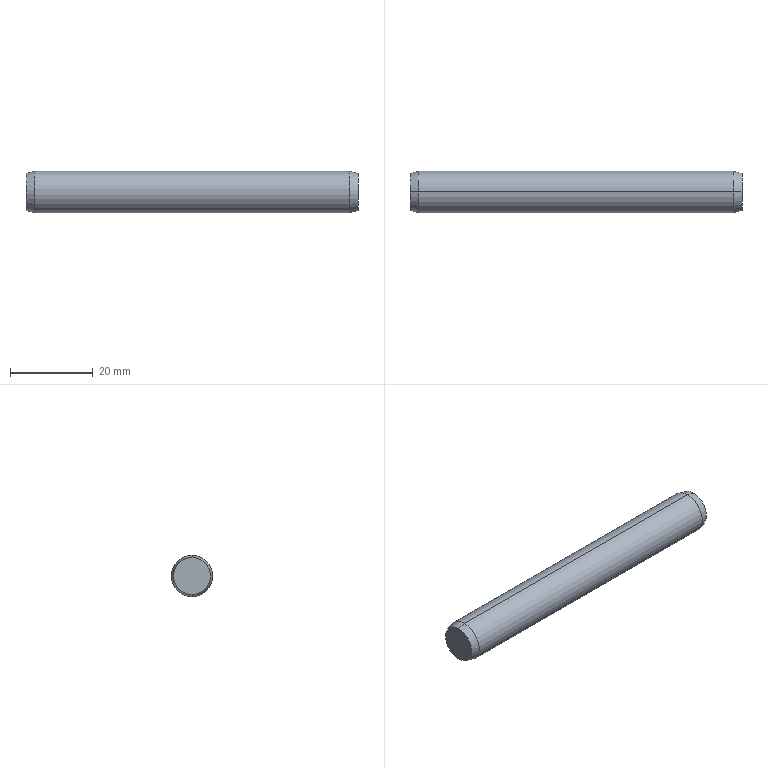Part | SolidWorks | features Revolution 1 | 1 solid | 8 faces | box 80 x 10 x 10 mm | volume 6251 mm3 | cone 4 | cylinder 2 | plane 2 | commonest cylinder face diameters 10 x2
STEP:
#1=CARTESIAN_POINT('',(0.,0.,-4.464));
#2=VERTEX_POINT('',#1);
#3=CARTESIAN_POINT('',(0.,0.,4.464));
#4=VERTEX_POINT('',#3);
#5=CARTESIAN_POINT('',(0.,0.,0.));
#6=DIRECTION('',(1.,0.,0.));
#7=DIRECTION('',(0.,0.,-1.));
#8=AXIS2_PLACEMENT_3D('',#5,#6,#7);
#9=CIRCLE('',#8,4.464);
#10=EDGE_CURVE('',#2,#4,#9,.T.);
#11=ORIENTED_EDGE('',*,*,#10,.T.);
#12=CARTESIAN_POINT('',(2.,0.,5.));
#13=VERTEX_POINT('',#12);
#14=CARTESIAN_POINT('',(2.,0.,5.));
#15=DIRECTION('',(0.9659,0.,0.2588));
#16=VECTOR('',#15,1000.);
#17=LINE('',#14,#16);
#18=EDGE_CURVE('',#4,#13,#17,.T.);
#19=ORIENTED_EDGE('',*,*,#18,.T.);
#20=CARTESIAN_POINT('',(2.,0.,-5.));
#21=VERTEX_POINT('',#20);
#22=CARTESIAN_POINT('',(2.,0.,0.));
#23=DIRECTION('',(1.,0.,0.));
#24=DIRECTION('',(0.,0.,-1.));
#25=AXIS2_PLACEMENT_3D('',#22,#23,#24);
#26=CIRCLE('',#25,5.);
#27=EDGE_CURVE('',#21,#13,#26,.T.);
#28=ORIENTED_EDGE('',*,*,#27,.F.);
#29=CARTESIAN_POINT('',(2.,0.,-5.));
#30=DIRECTION('',(0.9659,0.,-0.2588));
#31=VECTOR('',#30,1000.);
#32=LINE('',#29,#31);
#33=EDGE_CURVE('',#2,#21,#32,.T.);
#34=ORIENTED_EDGE('',*,*,#33,.F.);
#35=EDGE_LOOP('',(#11,#19,#28,#34));
#36=FACE_OUTER_BOUND('',#35,.T.);
#37=CARTESIAN_POINT('',(2.,0.,0.));
#38=DIRECTION('',(1.,0.,0.));
#39=DIRECTION('',(0.,0.,-1.));
#40=AXIS2_PLACEMENT_3D('',#37,#38,#39);
#41=CONICAL_SURFACE('',#40,5.,0.2618);
#42=ADVANCED_FACE('',(#36),#41,.T.);
#43=ORIENTED_EDGE('',*,*,#27,.T.);
#44=CARTESIAN_POINT('',(78.,0.,5.));
#45=VERTEX_POINT('',#44);
#46=CARTESIAN_POINT('',(0.,0.,5.));
#47=DIRECTION('',(1.,0.,0.));
#48=VECTOR('',#47,1000.);
#49=LINE('',#46,#48);
#50=EDGE_CURVE('',#13,#45,#49,.T.);
#51=ORIENTED_EDGE('',*,*,#50,.T.);
#52=CARTESIAN_POINT('',(78.,0.,-5.));
#53=VERTEX_POINT('',#52);
#54=CARTESIAN_POINT('',(78.,0.,0.));
#55=DIRECTION('',(1.,0.,0.));
#56=DIRECTION('',(0.,0.,-1.));
#57=AXIS2_PLACEMENT_3D('',#54,#55,#56);
#58=CIRCLE('',#57,5.);
#59=EDGE_CURVE('',#53,#45,#58,.T.);
#60=ORIENTED_EDGE('',*,*,#59,.F.);
#61=CARTESIAN_POINT('',(0.,0.,-5.));
#62=DIRECTION('',(1.,0.,0.));
#63=VECTOR('',#62,1000.);
#64=LINE('',#61,#63);
#65=EDGE_CURVE('',#21,#53,#64,.T.);
#66=ORIENTED_EDGE('',*,*,#65,.F.);
#67=EDGE_LOOP('',(#43,#51,#60,#66));
#68=FACE_OUTER_BOUND('',#67,.T.);
#69=CARTESIAN_POINT('',(0.,0.,0.));
#70=DIRECTION('',(1.,0.,0.));
#71=DIRECTION('',(0.,0.,-1.));
#72=AXIS2_PLACEMENT_3D('',#69,#70,#71);
#73=CYLINDRICAL_SURFACE('',#72,5.);
#74=ADVANCED_FACE('',(#68),#73,.T.);
#75=CARTESIAN_POINT('',(80.,0.,-4.464));
#76=VERTEX_POINT('',#75);
#77=CARTESIAN_POINT('',(80.,0.,4.464));
#78=VERTEX_POINT('',#77);
#79=CARTESIAN_POINT('',(80.,0.,0.));
#80=DIRECTION('',(1.,0.,0.));
#81=DIRECTION('',(0.,0.,-1.));
#82=AXIS2_PLACEMENT_3D('',#79,#80,#81);
#83=CIRCLE('',#82,4.464);
#84=EDGE_CURVE('',#76,#78,#83,.T.);
#85=ORIENTED_EDGE('',*,*,#84,.F.);
#86=CARTESIAN_POINT('',(80.,0.,-4.464));
#87=DIRECTION('',(-0.9659,0.,-0.2588));
#88=VECTOR('',#87,1000.);
#89=LINE('',#86,#88);
#90=EDGE_CURVE('',#76,#53,#89,.T.);
#91=ORIENTED_EDGE('',*,*,#90,.T.);
#92=ORIENTED_EDGE('',*,*,#59,.T.);
#93=CARTESIAN_POINT('',(80.,0.,4.464));
#94=DIRECTION('',(-0.9659,0.,0.2588));
#95=VECTOR('',#94,1000.);
#96=LINE('',#93,#95);
#97=EDGE_CURVE('',#78,#45,#96,.T.);
#98=ORIENTED_EDGE('',*,*,#97,.F.);
#99=EDGE_LOOP('',(#85,#91,#92,#98));
#100=FACE_OUTER_BOUND('',#99,.T.);
#101=CARTESIAN_POINT('',(80.,0.,0.));
#102=DIRECTION('',(-1.,0.,0.));
#103=DIRECTION('',(0.,0.,1.));
#104=AXIS2_PLACEMENT_3D('',#101,#102,#103);
#105=CONICAL_SURFACE('',#104,4.464,0.2618);
#106=ADVANCED_FACE('',(#100),#105,.T.);
#107=ORIENTED_EDGE('',*,*,#10,.F.);
#108=CARTESIAN_POINT('',(0.,0.,0.));
#109=DIRECTION('',(1.,0.,0.));
#110=DIRECTION('',(0.,0.,-1.));
#111=AXIS2_PLACEMENT_3D('',#108,#109,#110);
#112=CIRCLE('',#111,4.464);
#113=EDGE_CURVE('',#4,#2,#112,.T.);
#114=ORIENTED_EDGE('',*,*,#113,.F.);
#115=EDGE_LOOP('',(#107,#114));
#116=FACE_OUTER_BOUND('',#115,.T.);
#117=CARTESIAN_POINT('',(0.,4.464,0.));
#118=DIRECTION('',(-1.,0.,0.));
#119=DIRECTION('',(0.,0.,1.));
#120=AXIS2_PLACEMENT_3D('',#117,#118,#119);
#121=PLANE('',#120);
#122=ADVANCED_FACE('',(#116),#121,.T.);
#123=CARTESIAN_POINT('',(80.,0.,0.));
#124=DIRECTION('',(1.,0.,0.));
#125=DIRECTION('',(0.,0.,-1.));
#126=AXIS2_PLACEMENT_3D('',#123,#124,#125);
#127=CIRCLE('',#126,4.464);
#128=EDGE_CURVE('',#78,#76,#127,.T.);
#129=ORIENTED_EDGE('',*,*,#128,.T.);
#130=ORIENTED_EDGE('',*,*,#84,.T.);
#131=EDGE_LOOP('',(#129,#130));
#132=FACE_OUTER_BOUND('',#131,.T.);
#133=CARTESIAN_POINT('',(80.,4.464,0.));
#134=DIRECTION('',(1.,0.,0.));
#135=DIRECTION('',(0.,0.,-1.));
#136=AXIS2_PLACEMENT_3D('',#133,#134,#135);
#137=PLANE('',#136);
#138=ADVANCED_FACE('',(#132),#137,.T.);
#139=ORIENTED_EDGE('',*,*,#90,.F.);
#140=ORIENTED_EDGE('',*,*,#128,.F.);
#141=ORIENTED_EDGE('',*,*,#97,.T.);
#142=CARTESIAN_POINT('',(78.,0.,0.));
#143=DIRECTION('',(1.,0.,0.));
#144=DIRECTION('',(0.,0.,-1.));
#145=AXIS2_PLACEMENT_3D('',#142,#143,#144);
#146=CIRCLE('',#145,5.);
#147=EDGE_CURVE('',#45,#53,#146,.T.);
#148=ORIENTED_EDGE('',*,*,#147,.T.);
#149=EDGE_LOOP('',(#139,#140,#141,#148));
#150=FACE_OUTER_BOUND('',#149,.T.);
#151=CARTESIAN_POINT('',(80.,0.,0.));
#152=DIRECTION('',(-1.,0.,0.));
#153=DIRECTION('',(0.,0.,1.));
#154=AXIS2_PLACEMENT_3D('',#151,#152,#153);
#155=CONICAL_SURFACE('',#154,4.464,0.2618);
#156=ADVANCED_FACE('',(#150),#155,.T.);
#157=ORIENTED_EDGE('',*,*,#50,.F.);
#158=CARTESIAN_POINT('',(2.,0.,0.));
#159=DIRECTION('',(1.,0.,0.));
#160=DIRECTION('',(0.,0.,-1.));
#161=AXIS2_PLACEMENT_3D('',#158,#159,#160);
#162=CIRCLE('',#161,5.);
#163=EDGE_CURVE('',#13,#21,#162,.T.);
#164=ORIENTED_EDGE('',*,*,#163,.T.);
#165=ORIENTED_EDGE('',*,*,#65,.T.);
#166=ORIENTED_EDGE('',*,*,#147,.F.);
#167=EDGE_LOOP('',(#157,#164,#165,#166));
#168=FACE_OUTER_BOUND('',#167,.T.);
#169=CARTESIAN_POINT('',(0.,0.,0.));
#170=DIRECTION('',(1.,0.,0.));
#171=DIRECTION('',(0.,0.,-1.));
#172=AXIS2_PLACEMENT_3D('',#169,#170,#171);
#173=CYLINDRICAL_SURFACE('',#172,5.);
#174=ADVANCED_FACE('',(#168),#173,.T.);
#175=ORIENTED_EDGE('',*,*,#18,.F.);
#176=ORIENTED_EDGE('',*,*,#113,.T.);
#177=ORIENTED_EDGE('',*,*,#33,.T.);
#178=ORIENTED_EDGE('',*,*,#163,.F.);
#179=EDGE_LOOP('',(#175,#176,#177,#178));
#180=FACE_OUTER_BOUND('',#179,.T.);
#181=CARTESIAN_POINT('',(2.,0.,0.));
#182=DIRECTION('',(1.,0.,0.));
#183=DIRECTION('',(0.,0.,-1.));
#184=AXIS2_PLACEMENT_3D('',#181,#182,#183);
#185=CONICAL_SURFACE('',#184,5.,0.2618);
#186=ADVANCED_FACE('',(#180),#185,.T.);
#187=CLOSED_SHELL('',(#42,#74,#106,#122,#138,#156,#174,#186));
#188=MANIFOLD_SOLID_BREP('',#187);
#189=CARTESIAN_POINT('',(0.,0.,0.));
#190=DIRECTION('',(0.,0.,1.));
#191=DIRECTION('',(1.,0.,0.));
#192=AXIS2_PLACEMENT_3D('',#189,#190,#191);
#193=(LENGTH_UNIT()NAMED_UNIT(*)SI_UNIT(.MILLI.,.METRE.));
#194=UNCERTAINTY_MEASURE_WITH_UNIT(LENGTH_MEASURE(0.00001),#193,'','');
#195=(NAMED_UNIT(*)PLANE_ANGLE_UNIT()SI_UNIT($,.RADIAN.));
#196=(NAMED_UNIT(*)SI_UNIT($,.STERADIAN.)SOLID_ANGLE_UNIT());
#197=(GEOMETRIC_REPRESENTATION_CONTEXT(3)GLOBAL_UNCERTAINTY_ASSIGNED_CONTEXT((#194))GLOBAL_UNIT_ASSIGNED_CONTEXT((#193,#195,#196))REPRESENTATION_CONTEXT('',''));
#198=ADVANCED_BREP_SHAPE_REPRESENTATION('',(#188,#192),#197);